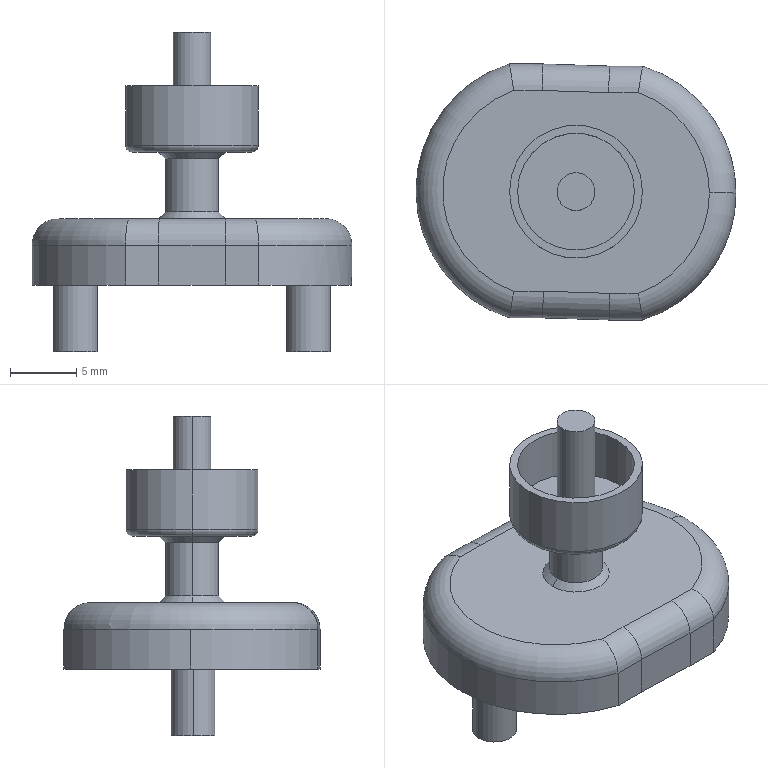Part | SolidWorks | features ICE 5, Fillet 2, Chamfer 1, Extrusion 1 | 1 solid | 44 faces | box 24.068 x 19.259 x 24 mm | volume 2234 mm3 | cylinder 21 | plane 14 | torus 5 | cone 4 | commonest cylinder face diameters 4 x8 3.305 x4 20 x3 2.85 x2 8.8 x2 10 x2
STEP:
#1=CARTESIAN_POINT('',(-1.721,5.002,10.));
#2=VERTEX_POINT('',#1);
#3=CARTESIAN_POINT('',(7.279,5.002,10.));
#4=VERTEX_POINT('',#3);
#5=CARTESIAN_POINT('',(2.779,5.002,10.));
#6=DIRECTION('',(0.,0.,-1.));
#7=DIRECTION('',(1.,0.,0.));
#8=AXIS2_PLACEMENT_3D('',#5,#6,#7);
#9=CIRCLE('',#8,4.5);
#10=EDGE_CURVE('',#2,#4,#9,.T.);
#11=ORIENTED_EDGE('',*,*,#10,.F.);
#12=CARTESIAN_POINT('',(-2.221,5.002,10.5));
#13=VERTEX_POINT('',#12);
#14=CARTESIAN_POINT('',(-1.721,5.002,10.5));
#15=DIRECTION('',(0.,1.,0.));
#16=DIRECTION('',(-1.,0.,0.));
#17=AXIS2_PLACEMENT_3D('',#14,#15,#16);
#18=CIRCLE('',#17,0.5);
#19=EDGE_CURVE('',#2,#13,#18,.T.);
#20=ORIENTED_EDGE('',*,*,#19,.T.);
#21=CARTESIAN_POINT('',(7.779,5.002,10.5));
#22=VERTEX_POINT('',#21);
#23=CARTESIAN_POINT('',(2.779,5.002,10.5));
#24=DIRECTION('',(0.,0.,1.));
#25=DIRECTION('',(1.,0.,0.));
#26=AXIS2_PLACEMENT_3D('',#23,#24,#25);
#27=CIRCLE('',#26,5.);
#28=EDGE_CURVE('',#22,#13,#27,.T.);
#29=ORIENTED_EDGE('',*,*,#28,.F.);
#30=CARTESIAN_POINT('',(7.279,5.002,10.5));
#31=DIRECTION('',(0.,-1.,0.));
#32=DIRECTION('',(0.,0.,-1.));
#33=AXIS2_PLACEMENT_3D('',#30,#31,#32);
#34=CIRCLE('',#33,0.5);
#35=EDGE_CURVE('',#4,#22,#34,.T.);
#36=ORIENTED_EDGE('',*,*,#35,.F.);
#37=EDGE_LOOP('',(#11,#20,#29,#36));
#38=FACE_OUTER_BOUND('',#37,.T.);
#39=CARTESIAN_POINT('',(2.779,5.002,10.5));
#40=DIRECTION('',(0.,0.,1.));
#41=DIRECTION('',(1.,0.,0.));
#42=AXIS2_PLACEMENT_3D('',#39,#40,#41);
#43=TOROIDAL_SURFACE('',#42,4.5,0.5);
#44=ADVANCED_FACE('',(#38),#43,.T.);
#45=CARTESIAN_POINT('',(4.779,5.002,5.5));
#46=VERTEX_POINT('',#45);
#47=CARTESIAN_POINT('',(0.7788,5.002,5.5));
#48=VERTEX_POINT('',#47);
#49=CARTESIAN_POINT('',(2.779,5.002,5.5));
#50=DIRECTION('',(0.,0.,1.));
#51=DIRECTION('',(1.,0.,0.));
#52=AXIS2_PLACEMENT_3D('',#49,#50,#51);
#53=CIRCLE('',#52,2.);
#54=EDGE_CURVE('',#46,#48,#53,.T.);
#55=ORIENTED_EDGE('',*,*,#54,.F.);
#56=CARTESIAN_POINT('',(5.279,5.002,5.));
#57=VERTEX_POINT('',#56);
#58=CARTESIAN_POINT('',(4.779,5.002,5.5));
#59=DIRECTION('',(0.7071,0.,-0.7071));
#60=VECTOR('',#59,1000.);
#61=LINE('',#58,#60);
#62=EDGE_CURVE('',#46,#57,#61,.T.);
#63=ORIENTED_EDGE('',*,*,#62,.T.);
#64=CARTESIAN_POINT('',(0.2788,5.002,5.));
#65=VERTEX_POINT('',#64);
#66=CARTESIAN_POINT('',(2.779,5.002,5.));
#67=DIRECTION('',(0.,0.,-1.));
#68=DIRECTION('',(1.,0.,0.));
#69=AXIS2_PLACEMENT_3D('',#66,#67,#68);
#70=CIRCLE('',#69,2.5);
#71=EDGE_CURVE('',#65,#57,#70,.T.);
#72=ORIENTED_EDGE('',*,*,#71,.F.);
#73=CARTESIAN_POINT('',(0.7788,5.002,5.5));
#74=DIRECTION('',(-0.7071,0.,-0.7071));
#75=VECTOR('',#74,1000.);
#76=LINE('',#73,#75);
#77=EDGE_CURVE('',#48,#65,#76,.T.);
#78=ORIENTED_EDGE('',*,*,#77,.F.);
#79=EDGE_LOOP('',(#55,#63,#72,#78));
#80=FACE_OUTER_BOUND('',#79,.T.);
#81=CARTESIAN_POINT('',(2.779,5.002,5.5));
#82=DIRECTION('',(0.,0.,-1.));
#83=DIRECTION('',(-1.,0.,0.));
#84=AXIS2_PLACEMENT_3D('',#81,#82,#83);
#85=CONICAL_SURFACE('',#84,2.,0.7854);
#86=ADVANCED_FACE('',(#80),#85,.T.);
#87=CARTESIAN_POINT('',(0.7788,5.002,9.5));
#88=VERTEX_POINT('',#87);
#89=CARTESIAN_POINT('',(4.779,5.002,9.5));
#90=VERTEX_POINT('',#89);
#91=CARTESIAN_POINT('',(2.779,5.002,9.5));
#92=DIRECTION('',(0.,0.,-1.));
#93=DIRECTION('',(1.,0.,0.));
#94=AXIS2_PLACEMENT_3D('',#91,#92,#93);
#95=CIRCLE('',#94,2.);
#96=EDGE_CURVE('',#88,#90,#95,.T.);
#97=ORIENTED_EDGE('',*,*,#96,.F.);
#98=CARTESIAN_POINT('',(0.2788,5.002,10.));
#99=VERTEX_POINT('',#98);
#100=CARTESIAN_POINT('',(0.2788,5.002,10.));
#101=DIRECTION('',(-0.7071,0.,0.7071));
#102=VECTOR('',#101,1000.);
#103=LINE('',#100,#102);
#104=EDGE_CURVE('',#88,#99,#103,.T.);
#105=ORIENTED_EDGE('',*,*,#104,.T.);
#106=CARTESIAN_POINT('',(5.279,5.002,10.));
#107=VERTEX_POINT('',#106);
#108=CARTESIAN_POINT('',(2.779,5.002,10.));
#109=DIRECTION('',(0.,0.,1.));
#110=DIRECTION('',(1.,0.,0.));
#111=AXIS2_PLACEMENT_3D('',#108,#109,#110);
#112=CIRCLE('',#111,2.5);
#113=EDGE_CURVE('',#107,#99,#112,.T.);
#114=ORIENTED_EDGE('',*,*,#113,.F.);
#115=CARTESIAN_POINT('',(5.279,5.002,10.));
#116=DIRECTION('',(0.7071,0.,0.7071));
#117=VECTOR('',#116,1000.);
#118=LINE('',#115,#117);
#119=EDGE_CURVE('',#90,#107,#118,.T.);
#120=ORIENTED_EDGE('',*,*,#119,.F.);
#121=EDGE_LOOP('',(#97,#105,#114,#120));
#122=FACE_OUTER_BOUND('',#121,.T.);
#123=CARTESIAN_POINT('',(2.779,5.002,10.));
#124=DIRECTION('',(0.,0.,1.));
#125=DIRECTION('',(1.,0.,0.));
#126=AXIS2_PLACEMENT_3D('',#123,#124,#125);
#127=CONICAL_SURFACE('',#126,2.5,0.7854);
#128=ADVANCED_FACE('',(#122),#127,.T.);
#129=CARTESIAN_POINT('',(4.204,5.002,19.));
#130=VERTEX_POINT('',#129);
#131=CARTESIAN_POINT('',(1.354,5.002,19.));
#132=VERTEX_POINT('',#131);
#133=CARTESIAN_POINT('',(2.779,5.002,19.));
#134=DIRECTION('',(0.,0.,1.));
#135=DIRECTION('',(1.,0.,0.));
#136=AXIS2_PLACEMENT_3D('',#133,#134,#135);
#137=CIRCLE('',#136,1.425);
#138=EDGE_CURVE('',#130,#132,#137,.T.);
#139=ORIENTED_EDGE('',*,*,#138,.F.);
#140=CARTESIAN_POINT('',(4.204,5.002,11.));
#141=VERTEX_POINT('',#140);
#142=CARTESIAN_POINT('',(4.204,5.002,19.));
#143=DIRECTION('',(0.,0.,-1.));
#144=VECTOR('',#143,1000.);
#145=LINE('',#142,#144);
#146=EDGE_CURVE('',#130,#141,#145,.T.);
#147=ORIENTED_EDGE('',*,*,#146,.T.);
#148=CARTESIAN_POINT('',(1.354,5.002,11.));
#149=VERTEX_POINT('',#148);
#150=CARTESIAN_POINT('',(2.779,5.002,11.));
#151=DIRECTION('',(0.,0.,1.));
#152=DIRECTION('',(1.,0.,0.));
#153=AXIS2_PLACEMENT_3D('',#150,#151,#152);
#154=CIRCLE('',#153,1.425);
#155=EDGE_CURVE('',#141,#149,#154,.T.);
#156=ORIENTED_EDGE('',*,*,#155,.T.);
#157=CARTESIAN_POINT('',(1.354,5.002,19.));
#158=DIRECTION('',(0.,0.,-1.));
#159=VECTOR('',#158,1000.);
#160=LINE('',#157,#159);
#161=EDGE_CURVE('',#132,#149,#160,.T.);
#162=ORIENTED_EDGE('',*,*,#161,.F.);
#163=EDGE_LOOP('',(#139,#147,#156,#162));
#164=FACE_OUTER_BOUND('',#163,.T.);
#165=CARTESIAN_POINT('',(2.779,5.002,19.));
#166=DIRECTION('',(0.,0.,-1.));
#167=DIRECTION('',(-1.,0.,0.));
#168=AXIS2_PLACEMENT_3D('',#165,#166,#167);
#169=CYLINDRICAL_SURFACE('',#168,1.425);
#170=ADVANCED_FACE('',(#164),#169,.T.);
#171=CARTESIAN_POINT('',(-1.621,5.002,15.));
#172=VERTEX_POINT('',#171);
#173=CARTESIAN_POINT('',(7.179,5.002,15.));
#174=VERTEX_POINT('',#173);
#175=CARTESIAN_POINT('',(2.779,5.002,15.));
#176=DIRECTION('',(0.,0.,1.));
#177=DIRECTION('',(1.,0.,0.));
#178=AXIS2_PLACEMENT_3D('',#175,#176,#177);
#179=CIRCLE('',#178,4.4);
#180=EDGE_CURVE('',#172,#174,#179,.T.);
#181=ORIENTED_EDGE('',*,*,#180,.T.);
#182=CARTESIAN_POINT('',(7.179,5.002,11.));
#183=VERTEX_POINT('',#182);
#184=CARTESIAN_POINT('',(7.179,5.002,15.));
#185=DIRECTION('',(0.,0.,-1.));
#186=VECTOR('',#185,1000.);
#187=LINE('',#184,#186);
#188=EDGE_CURVE('',#174,#183,#187,.T.);
#189=ORIENTED_EDGE('',*,*,#188,.T.);
#190=CARTESIAN_POINT('',(-1.621,5.002,11.));
#191=VERTEX_POINT('',#190);
#192=CARTESIAN_POINT('',(2.779,5.002,11.));
#193=DIRECTION('',(0.,0.,-1.));
#194=DIRECTION('',(1.,0.,0.));
#195=AXIS2_PLACEMENT_3D('',#192,#193,#194);
#196=CIRCLE('',#195,4.4);
#197=EDGE_CURVE('',#183,#191,#196,.T.);
#198=ORIENTED_EDGE('',*,*,#197,.T.);
#199=CARTESIAN_POINT('',(-1.621,5.002,15.));
#200=DIRECTION('',(0.,0.,-1.));
#201=VECTOR('',#200,1000.);
#202=LINE('',#199,#201);
#203=EDGE_CURVE('',#172,#191,#202,.T.);
#204=ORIENTED_EDGE('',*,*,#203,.F.);
#205=EDGE_LOOP('',(#181,#189,#198,#204));
#206=FACE_OUTER_BOUND('',#205,.T.);
#207=CARTESIAN_POINT('',(2.779,5.002,15.));
#208=DIRECTION('',(0.,0.,-1.));
#209=DIRECTION('',(-1.,0.,0.));
#210=AXIS2_PLACEMENT_3D('',#207,#208,#209);
#211=CYLINDRICAL_SURFACE('',#210,4.4);
#212=ADVANCED_FACE('',(#206),#211,.F.);
#213=CARTESIAN_POINT('',(7.779,5.002,15.));
#214=VERTEX_POINT('',#213);
#215=CARTESIAN_POINT('',(-2.221,5.002,15.));
#216=VERTEX_POINT('',#215);
#217=CARTESIAN_POINT('',(2.779,5.002,15.));
#218=DIRECTION('',(0.,0.,1.));
#219=DIRECTION('',(1.,0.,0.));
#220=AXIS2_PLACEMENT_3D('',#217,#218,#219);
#221=CIRCLE('',#220,5.);
#222=EDGE_CURVE('',#214,#216,#221,.T.);
#223=ORIENTED_EDGE('',*,*,#222,.F.);
#224=CARTESIAN_POINT('',(7.779,5.002,15.));
#225=DIRECTION('',(0.,0.,-1.));
#226=VECTOR('',#225,1000.);
#227=LINE('',#224,#226);
#228=EDGE_CURVE('',#214,#22,#227,.T.);
#229=ORIENTED_EDGE('',*,*,#228,.T.);
#230=ORIENTED_EDGE('',*,*,#28,.T.);
#231=CARTESIAN_POINT('',(-2.221,5.002,15.));
#232=DIRECTION('',(0.,0.,-1.));
#233=VECTOR('',#232,1000.);
#234=LINE('',#231,#233);
#235=EDGE_CURVE('',#216,#13,#234,.T.);
#236=ORIENTED_EDGE('',*,*,#235,.F.);
#237=EDGE_LOOP('',(#223,#229,#230,#236));
#238=FACE_OUTER_BOUND('',#237,.T.);
#239=CARTESIAN_POINT('',(2.779,5.002,15.));
#240=DIRECTION('',(0.,0.,-1.));
#241=DIRECTION('',(-1.,0.,0.));
#242=AXIS2_PLACEMENT_3D('',#239,#240,#241);
#243=CYLINDRICAL_SURFACE('',#242,5.);
#244=ADVANCED_FACE('',(#238),#243,.T.);
#245=ORIENTED_EDGE('',*,*,#96,.T.);
#246=CARTESIAN_POINT('',(4.779,5.002,10.));
#247=DIRECTION('',(0.,0.,-1.));
#248=VECTOR('',#247,1000.);
#249=LINE('',#246,#248);
#250=EDGE_CURVE('',#90,#46,#249,.T.);
#251=ORIENTED_EDGE('',*,*,#250,.T.);
#252=ORIENTED_EDGE('',*,*,#54,.T.);
#253=CARTESIAN_POINT('',(0.7788,5.002,10.));
#254=DIRECTION('',(0.,0.,-1.));
#255=VECTOR('',#254,1000.);
#256=LINE('',#253,#255);
#257=EDGE_CURVE('',#88,#48,#256,.T.);
#258=ORIENTED_EDGE('',*,*,#257,.F.);
#259=EDGE_LOOP('',(#245,#251,#252,#258));
#260=FACE_OUTER_BOUND('',#259,.T.);
#261=CARTESIAN_POINT('',(2.779,5.002,10.));
#262=DIRECTION('',(0.,0.,-1.));
#263=DIRECTION('',(-1.,0.,0.));
#264=AXIS2_PLACEMENT_3D('',#261,#262,#263);
#265=CYLINDRICAL_SURFACE('',#264,2.);
#266=ADVANCED_FACE('',(#260),#265,.T.);
#267=CARTESIAN_POINT('',(14.813,4.922,3.));
#268=VERTEX_POINT('',#267);
#269=CARTESIAN_POINT('',(7.779,-4.628,3.));
#270=VERTEX_POINT('',#269);
#271=CARTESIAN_POINT('',(4.813,4.922,3.));
#272=DIRECTION('',(0.,0.,-1.));
#273=DIRECTION('',(1.,0.,0.));
#274=AXIS2_PLACEMENT_3D('',#271,#272,#273);
#275=CIRCLE('',#274,10.);
#276=EDGE_CURVE('',#268,#270,#275,.T.);
#277=ORIENTED_EDGE('',*,*,#276,.F.);
#278=CARTESIAN_POINT('',(12.813,4.922,5.));
#279=VERTEX_POINT('',#278);
#280=CARTESIAN_POINT('',(12.813,4.922,3.));
#281=DIRECTION('',(0.,-1.,0.));
#282=DIRECTION('',(0.,0.,-1.));
#283=AXIS2_PLACEMENT_3D('',#280,#281,#282);
#284=CIRCLE('',#283,2.);
#285=EDGE_CURVE('',#268,#279,#284,.T.);
#286=ORIENTED_EDGE('',*,*,#285,.T.);
#287=CARTESIAN_POINT('',(7.458,-2.628,5.));
#288=VERTEX_POINT('',#287);
#289=CARTESIAN_POINT('',(4.813,4.922,5.));
#290=DIRECTION('',(0.,0.,1.));
#291=DIRECTION('',(1.,0.,0.));
#292=AXIS2_PLACEMENT_3D('',#289,#290,#291);
#293=CIRCLE('',#292,8.);
#294=EDGE_CURVE('',#288,#279,#293,.T.);
#295=ORIENTED_EDGE('',*,*,#294,.F.);
#296=CARTESIAN_POINT('',(7.779,-4.628,3.));
#297=CARTESIAN_POINT('',(7.779,-4.628,3.133));
#298=CARTESIAN_POINT('',(7.777,-4.614,3.264));
#299=CARTESIAN_POINT('',(7.769,-4.563,3.521));
#300=CARTESIAN_POINT('',(7.763,-4.524,3.648));
#301=CARTESIAN_POINT('',(7.748,-4.423,3.891));
#302=CARTESIAN_POINT('',(7.738,-4.361,4.006));
#303=CARTESIAN_POINT('',(7.716,-4.215,4.224));
#304=CARTESIAN_POINT('',(7.702,-4.13,4.327));
#305=CARTESIAN_POINT('',(7.659,-3.852,4.602));
#306=CARTESIAN_POINT('',(7.624,-3.629,4.75));
#307=CARTESIAN_POINT('',(7.546,-3.15,4.948));
#308=CARTESIAN_POINT('',(7.502,-2.886,5.));
#309=CARTESIAN_POINT('',(7.458,-2.628,5.));
#310=B_SPLINE_CURVE_WITH_KNOTS('',3,(#296,#297,#298,#299,#300,#301,#302,#303,#304,#305,#306,#307,#308,#309),.UNSPECIFIED.,.F.,.F.,(4,2,2,2,2,2,4),(0.,0.0003931,0.0007862,0.001179,0.001572,0.002359,0.003145),.UNSPECIFIED.);
#311=EDGE_CURVE('',#270,#288,#310,.T.);
#312=ORIENTED_EDGE('',*,*,#311,.F.);
#313=EDGE_LOOP('',(#277,#286,#295,#312));
#314=FACE_OUTER_BOUND('',#313,.T.);
#315=CARTESIAN_POINT('',(4.813,4.922,3.));
#316=DIRECTION('',(0.,0.,1.));
#317=DIRECTION('',(1.,0.,0.));
#318=AXIS2_PLACEMENT_3D('',#315,#316,#317);
#319=TOROIDAL_SURFACE('',#318,8.,2.);
#320=ADVANCED_FACE('',(#314),#319,.T.);
#321=CARTESIAN_POINT('',(-7.628,4.922,-5.));
#322=VERTEX_POINT('',#321);
#323=CARTESIAN_POINT('',(-4.323,4.922,-5.));
#324=VERTEX_POINT('',#323);
#325=CARTESIAN_POINT('',(-5.975,4.922,-5.));
#326=DIRECTION('',(0.,0.,-1.));
#327=DIRECTION('',(-1.,0.,0.));
#328=AXIS2_PLACEMENT_3D('',#325,#326,#327);
#329=CIRCLE('',#328,1.652);
#330=EDGE_CURVE('',#322,#324,#329,.T.);
#331=ORIENTED_EDGE('',*,*,#330,.F.);
#332=CARTESIAN_POINT('',(-7.628,4.922,0.));
#333=VERTEX_POINT('',#332);
#334=CARTESIAN_POINT('',(-7.628,4.922,-5.));
#335=DIRECTION('',(0.,0.,1.));
#336=VECTOR('',#335,1000.);
#337=LINE('',#334,#336);
#338=EDGE_CURVE('',#322,#333,#337,.T.);
#339=ORIENTED_EDGE('',*,*,#338,.T.);
#340=CARTESIAN_POINT('',(-4.323,4.922,0.));
#341=VERTEX_POINT('',#340);
#342=CARTESIAN_POINT('',(-5.975,4.922,0.));
#343=DIRECTION('',(0.,0.,-1.));
#344=DIRECTION('',(1.,0.,0.));
#345=AXIS2_PLACEMENT_3D('',#342,#343,#344);
#346=CIRCLE('',#345,1.652);
#347=EDGE_CURVE('',#333,#341,#346,.T.);
#348=ORIENTED_EDGE('',*,*,#347,.T.);
#349=CARTESIAN_POINT('',(-4.323,4.922,-5.));
#350=DIRECTION('',(0.,0.,1.));
#351=VECTOR('',#350,1000.);
#352=LINE('',#349,#351);
#353=EDGE_CURVE('',#324,#341,#352,.T.);
#354=ORIENTED_EDGE('',*,*,#353,.F.);
#355=EDGE_LOOP('',(#331,#339,#348,#354));
#356=FACE_OUTER_BOUND('',#355,.T.);
#357=CARTESIAN_POINT('',(-5.975,4.922,-5.));
#358=DIRECTION('',(0.,0.,1.));
#359=DIRECTION('',(1.,0.,0.));
#360=AXIS2_PLACEMENT_3D('',#357,#358,#359);
#361=CYLINDRICAL_SURFACE('',#360,1.652);
#362=ADVANCED_FACE('',(#356),#361,.T.);
#363=CARTESIAN_POINT('',(9.88,4.922,-5.));
#364=VERTEX_POINT('',#363);
#365=CARTESIAN_POINT('',(13.185,4.922,-5.));
#366=VERTEX_POINT('',#365);
#367=CARTESIAN_POINT('',(11.533,4.922,-5.));
#368=DIRECTION('',(0.,0.,-1.));
#369=DIRECTION('',(-1.,0.,0.));
#370=AXIS2_PLACEMENT_3D('',#367,#368,#369);
#371=CIRCLE('',#370,1.652);
#372=EDGE_CURVE('',#364,#366,#371,.T.);
#373=ORIENTED_EDGE('',*,*,#372,.F.);
#374=CARTESIAN_POINT('',(9.88,4.922,0.));
#375=VERTEX_POINT('',#374);
#376=CARTESIAN_POINT('',(9.88,4.922,-5.));
#377=DIRECTION('',(0.,0.,1.));
#378=VECTOR('',#377,1000.);
#379=LINE('',#376,#378);
#380=EDGE_CURVE('',#364,#375,#379,.T.);
#381=ORIENTED_EDGE('',*,*,#380,.T.);
#382=CARTESIAN_POINT('',(13.185,4.922,0.));
#383=VERTEX_POINT('',#382);
#384=CARTESIAN_POINT('',(11.533,4.922,0.));
#385=DIRECTION('',(0.,0.,-1.));
#386=DIRECTION('',(1.,0.,0.));
#387=AXIS2_PLACEMENT_3D('',#384,#385,#386);
#388=CIRCLE('',#387,1.652);
#389=EDGE_CURVE('',#375,#383,#388,.T.);
#390=ORIENTED_EDGE('',*,*,#389,.T.);
#391=CARTESIAN_POINT('',(13.185,4.922,-5.));
#392=DIRECTION('',(0.,0.,1.));
#393=VECTOR('',#392,1000.);
#394=LINE('',#391,#393);
#395=EDGE_CURVE('',#366,#383,#394,.T.);
#396=ORIENTED_EDGE('',*,*,#395,.F.);
#397=EDGE_LOOP('',(#373,#381,#390,#396));
#398=FACE_OUTER_BOUND('',#397,.T.);
#399=CARTESIAN_POINT('',(11.533,4.922,-5.));
#400=DIRECTION('',(0.,0.,1.));
#401=DIRECTION('',(1.,0.,0.));
#402=AXIS2_PLACEMENT_3D('',#399,#400,#401);
#403=CYLINDRICAL_SURFACE('',#402,1.652);
#404=ADVANCED_FACE('',(#398),#403,.T.);
#405=CARTESIAN_POINT('',(-2.221,-4.469,3.));
#406=VERTEX_POINT('',#405);
#407=CARTESIAN_POINT('',(-9.255,5.081,3.));
#408=VERTEX_POINT('',#407);
#409=CARTESIAN_POINT('',(0.7449,5.081,3.));
#410=DIRECTION('',(0.,0.,-1.));
#411=DIRECTION('',(1.,0.,0.));
#412=AXIS2_PLACEMENT_3D('',#409,#410,#411);
#413=CIRCLE('',#412,10.);
#414=EDGE_CURVE('',#406,#408,#413,.T.);
#415=ORIENTED_EDGE('',*,*,#414,.T.);
#416=CARTESIAN_POINT('',(-9.255,5.081,0.));
#417=VERTEX_POINT('',#416);
#418=CARTESIAN_POINT('',(-9.255,5.081,5.));
#419=DIRECTION('',(0.,0.,-1.));
#420=VECTOR('',#419,1000.);
#421=LINE('',#418,#420);
#422=EDGE_CURVE('',#408,#417,#421,.T.);
#423=ORIENTED_EDGE('',*,*,#422,.T.);
#424=CARTESIAN_POINT('',(-2.221,-4.469,0.));
#425=VERTEX_POINT('',#424);
#426=CARTESIAN_POINT('',(0.7449,5.081,0.));
#427=DIRECTION('',(0.,0.,1.));
#428=DIRECTION('',(1.,0.,0.));
#429=AXIS2_PLACEMENT_3D('',#426,#427,#428);
#430=CIRCLE('',#429,10.);
#431=EDGE_CURVE('',#417,#425,#430,.T.);
#432=ORIENTED_EDGE('',*,*,#431,.T.);
#433=CARTESIAN_POINT('',(-2.221,-4.469,5.));
#434=DIRECTION('',(0.,0.,-1.));
#435=VECTOR('',#434,1000.);
#436=LINE('',#433,#435);
#437=EDGE_CURVE('',#406,#425,#436,.T.);
#438=ORIENTED_EDGE('',*,*,#437,.F.);
#439=EDGE_LOOP('',(#415,#423,#432,#438));
#440=FACE_OUTER_BOUND('',#439,.T.);
#441=CARTESIAN_POINT('',(0.7449,5.081,5.));
#442=DIRECTION('',(0.,0.,-1.));
#443=DIRECTION('',(-1.,0.,0.));
#444=AXIS2_PLACEMENT_3D('',#441,#442,#443);
#445=CYLINDRICAL_SURFACE('',#444,10.);
#446=ADVANCED_FACE('',(#440),#445,.T.);
#447=CARTESIAN_POINT('',(0.2788,-4.469,3.));
#448=VERTEX_POINT('',#447);
#449=CARTESIAN_POINT('',(0.2788,-4.469,0.));
#450=VERTEX_POINT('',#449);
#451=CARTESIAN_POINT('',(0.2788,-4.469,5.));
#452=DIRECTION('',(0.,0.,-1.));
#453=VECTOR('',#452,1000.);
#454=LINE('',#451,#453);
#455=EDGE_CURVE('',#448,#450,#454,.T.);
#456=ORIENTED_EDGE('',*,*,#455,.F.);
#457=CARTESIAN_POINT('',(-2.221,-4.469,3.));
#458=DIRECTION('',(-1.,0.,0.));
#459=VECTOR('',#458,1000.);
#460=LINE('',#457,#459);
#461=EDGE_CURVE('',#448,#406,#460,.T.);
#462=ORIENTED_EDGE('',*,*,#461,.T.);
#463=ORIENTED_EDGE('',*,*,#437,.T.);
#464=CARTESIAN_POINT('',(-1.721,-4.469,0.));
#465=DIRECTION('',(1.,0.,0.));
#466=VECTOR('',#465,1000.);
#467=LINE('',#464,#466);
#468=EDGE_CURVE('',#425,#450,#467,.T.);
#469=ORIENTED_EDGE('',*,*,#468,.T.);
#470=EDGE_LOOP('',(#456,#462,#463,#469));
#471=FACE_OUTER_BOUND('',#470,.T.);
#472=CARTESIAN_POINT('',(-1.721,-4.469,5.));
#473=DIRECTION('',(0.,1.,0.));
#474=DIRECTION('',(0.,0.,1.));
#475=AXIS2_PLACEMENT_3D('',#472,#473,#474);
#476=PLANE('',#475);
#477=ADVANCED_FACE('',(#471),#476,.F.);
#478=CARTESIAN_POINT('',(5.279,-4.628,3.));
#479=VERTEX_POINT('',#478);
#480=CARTESIAN_POINT('',(5.279,-4.628,0.));
#481=VERTEX_POINT('',#480);
#482=CARTESIAN_POINT('',(5.279,-4.628,5.));
#483=DIRECTION('',(0.,0.,-1.));
#484=VECTOR('',#483,1000.);
#485=LINE('',#482,#484);
#486=EDGE_CURVE('',#479,#481,#485,.T.);
#487=ORIENTED_EDGE('',*,*,#486,.F.);
#488=CARTESIAN_POINT('',(0.2788,-4.469,3.));
#489=DIRECTION('',(-0.9995,0.03174,0.));
#490=VECTOR('',#489,1000.);
#491=LINE('',#488,#490);
#492=EDGE_CURVE('',#479,#448,#491,.T.);
#493=ORIENTED_EDGE('',*,*,#492,.T.);
#494=ORIENTED_EDGE('',*,*,#455,.T.);
#495=CARTESIAN_POINT('',(5.279,-4.628,0.));
#496=DIRECTION('',(0.9995,-0.03174,0.));
#497=VECTOR('',#496,1000.);
#498=LINE('',#495,#497);
#499=EDGE_CURVE('',#450,#481,#498,.T.);
#500=ORIENTED_EDGE('',*,*,#499,.T.);
#501=EDGE_LOOP('',(#487,#493,#494,#500));
#502=FACE_OUTER_BOUND('',#501,.T.);
#503=CARTESIAN_POINT('',(5.279,-4.628,5.));
#504=DIRECTION('',(0.03174,0.9995,0.));
#505=DIRECTION('',(-0.9995,0.03174,0.));
#506=AXIS2_PLACEMENT_3D('',#503,#504,#505);
#507=PLANE('',#506);
#508=ADVANCED_FACE('',(#502),#507,.F.);
#509=CARTESIAN_POINT('',(7.779,-4.628,0.));
#510=VERTEX_POINT('',#509);
#511=CARTESIAN_POINT('',(7.779,-4.628,5.));
#512=DIRECTION('',(0.,0.,-1.));
#513=VECTOR('',#512,1000.);
#514=LINE('',#511,#513);
#515=EDGE_CURVE('',#270,#510,#514,.T.);
#516=ORIENTED_EDGE('',*,*,#515,.F.);
#517=CARTESIAN_POINT('',(5.279,-4.628,3.));
#518=DIRECTION('',(-1.,0.,0.));
#519=VECTOR('',#518,1000.);
#520=LINE('',#517,#519);
#521=EDGE_CURVE('',#270,#479,#520,.T.);
#522=ORIENTED_EDGE('',*,*,#521,.T.);
#523=ORIENTED_EDGE('',*,*,#486,.T.);
#524=CARTESIAN_POINT('',(7.779,-4.628,0.));
#525=DIRECTION('',(1.,0.,0.));
#526=VECTOR('',#525,1000.);
#527=LINE('',#524,#526);
#528=EDGE_CURVE('',#481,#510,#527,.T.);
#529=ORIENTED_EDGE('',*,*,#528,.T.);
#530=EDGE_LOOP('',(#516,#522,#523,#529));
#531=FACE_OUTER_BOUND('',#530,.T.);
#532=CARTESIAN_POINT('',(7.779,-4.628,5.));
#533=DIRECTION('',(0.,1.,0.));
#534=DIRECTION('',(0.,0.,1.));
#535=AXIS2_PLACEMENT_3D('',#532,#533,#534);
#536=PLANE('',#535);
#537=ADVANCED_FACE('',(#531),#536,.F.);
#538=CARTESIAN_POINT('',(7.779,14.472,3.));
#539=VERTEX_POINT('',#538);
#540=CARTESIAN_POINT('',(7.779,14.472,0.));
#541=VERTEX_POINT('',#540);
#542=CARTESIAN_POINT('',(7.779,14.472,5.));
#543=DIRECTION('',(0.,0.,-1.));
#544=VECTOR('',#543,1000.);
#545=LINE('',#542,#544);
#546=EDGE_CURVE('',#539,#541,#545,.T.);
#547=ORIENTED_EDGE('',*,*,#546,.F.);
#548=CARTESIAN_POINT('',(4.813,4.922,3.));
#549=DIRECTION('',(0.,0.,-1.));
#550=DIRECTION('',(1.,0.,0.));
#551=AXIS2_PLACEMENT_3D('',#548,#549,#550);
#552=CIRCLE('',#551,10.);
#553=EDGE_CURVE('',#539,#268,#552,.T.);
#554=ORIENTED_EDGE('',*,*,#553,.T.);
#555=ORIENTED_EDGE('',*,*,#276,.T.);
#556=ORIENTED_EDGE('',*,*,#515,.T.);
#557=CARTESIAN_POINT('',(4.813,4.922,0.));
#558=DIRECTION('',(0.,0.,1.));
#559=DIRECTION('',(1.,0.,0.));
#560=AXIS2_PLACEMENT_3D('',#557,#558,#559);
#561=CIRCLE('',#560,10.);
#562=EDGE_CURVE('',#510,#541,#561,.T.);
#563=ORIENTED_EDGE('',*,*,#562,.T.);
#564=EDGE_LOOP('',(#547,#554,#555,#556,#563));
#565=FACE_OUTER_BOUND('',#564,.T.);
#566=CARTESIAN_POINT('',(4.813,4.922,5.));
#567=DIRECTION('',(0.,0.,-1.));
#568=DIRECTION('',(-1.,0.,0.));
#569=AXIS2_PLACEMENT_3D('',#566,#567,#568);
#570=CYLINDRICAL_SURFACE('',#569,10.);
#571=ADVANCED_FACE('',(#565),#570,.T.);
#572=CARTESIAN_POINT('',(5.279,14.472,3.));
#573=VERTEX_POINT('',#572);
#574=CARTESIAN_POINT('',(5.279,14.472,0.));
#575=VERTEX_POINT('',#574);
#576=CARTESIAN_POINT('',(5.279,14.472,5.));
#577=DIRECTION('',(0.,0.,-1.));
#578=VECTOR('',#577,1000.);
#579=LINE('',#576,#578);
#580=EDGE_CURVE('',#573,#575,#579,.T.);
#581=ORIENTED_EDGE('',*,*,#580,.F.);
#582=CARTESIAN_POINT('',(7.779,14.472,3.));
#583=DIRECTION('',(1.,0.,0.));
#584=VECTOR('',#583,1000.);
#585=LINE('',#582,#584);
#586=EDGE_CURVE('',#573,#539,#585,.T.);
#587=ORIENTED_EDGE('',*,*,#586,.T.);
#588=ORIENTED_EDGE('',*,*,#546,.T.);
#589=CARTESIAN_POINT('',(7.279,14.472,0.));
#590=DIRECTION('',(-1.,0.,0.));
#591=VECTOR('',#590,1000.);
#592=LINE('',#589,#591);
#593=EDGE_CURVE('',#541,#575,#592,.T.);
#594=ORIENTED_EDGE('',*,*,#593,.T.);
#595=EDGE_LOOP('',(#581,#587,#588,#594));
#596=FACE_OUTER_BOUND('',#595,.T.);
#597=CARTESIAN_POINT('',(7.279,14.472,5.));
#598=DIRECTION('',(0.,-1.,0.));
#599=DIRECTION('',(0.,0.,-1.));
#600=AXIS2_PLACEMENT_3D('',#597,#598,#599);
#601=PLANE('',#600);
#602=ADVANCED_FACE('',(#596),#601,.F.);
#603=CARTESIAN_POINT('',(0.2788,14.631,3.));
#604=VERTEX_POINT('',#603);
#605=CARTESIAN_POINT('',(0.2788,14.631,0.));
#606=VERTEX_POINT('',#605);
#607=CARTESIAN_POINT('',(0.2788,14.631,5.));
#608=DIRECTION('',(0.,0.,-1.));
#609=VECTOR('',#608,1000.);
#610=LINE('',#607,#609);
#611=EDGE_CURVE('',#604,#606,#610,.T.);
#612=ORIENTED_EDGE('',*,*,#611,.F.);
#613=CARTESIAN_POINT('',(5.279,14.472,3.));
#614=DIRECTION('',(0.9995,-0.03174,0.));
#615=VECTOR('',#614,1000.);
#616=LINE('',#613,#615);
#617=EDGE_CURVE('',#604,#573,#616,.T.);
#618=ORIENTED_EDGE('',*,*,#617,.T.);
#619=ORIENTED_EDGE('',*,*,#580,.T.);
#620=CARTESIAN_POINT('',(0.2788,14.631,0.));
#621=DIRECTION('',(-0.9995,0.03174,0.));
#622=VECTOR('',#621,1000.);
#623=LINE('',#620,#622);
#624=EDGE_CURVE('',#575,#606,#623,.T.);
#625=ORIENTED_EDGE('',*,*,#624,.T.);
#626=EDGE_LOOP('',(#612,#618,#619,#625));
#627=FACE_OUTER_BOUND('',#626,.T.);
#628=CARTESIAN_POINT('',(0.2788,14.631,5.));
#629=DIRECTION('',(-0.03174,-0.9995,0.));
#630=DIRECTION('',(0.9995,-0.03174,0.));
#631=AXIS2_PLACEMENT_3D('',#628,#629,#630);
#632=PLANE('',#631);
#633=ADVANCED_FACE('',(#627),#632,.F.);
#634=CARTESIAN_POINT('',(-2.221,14.631,3.));
#635=VERTEX_POINT('',#634);
#636=CARTESIAN_POINT('',(-2.221,14.631,0.));
#637=VERTEX_POINT('',#636);
#638=CARTESIAN_POINT('',(-2.221,14.631,5.));
#639=DIRECTION('',(0.,0.,-1.));
#640=VECTOR('',#639,1000.);
#641=LINE('',#638,#640);
#642=EDGE_CURVE('',#635,#637,#641,.T.);
#643=ORIENTED_EDGE('',*,*,#642,.F.);
#644=CARTESIAN_POINT('',(0.2788,14.631,3.));
#645=DIRECTION('',(1.,0.,0.));
#646=VECTOR('',#645,1000.);
#647=LINE('',#644,#646);
#648=EDGE_CURVE('',#635,#604,#647,.T.);
#649=ORIENTED_EDGE('',*,*,#648,.T.);
#650=ORIENTED_EDGE('',*,*,#611,.T.);
#651=CARTESIAN_POINT('',(-2.221,14.631,0.));
#652=DIRECTION('',(-1.,0.,0.));
#653=VECTOR('',#652,1000.);
#654=LINE('',#651,#653);
#655=EDGE_CURVE('',#606,#637,#654,.T.);
#656=ORIENTED_EDGE('',*,*,#655,.T.);
#657=EDGE_LOOP('',(#643,#649,#650,#656));
#658=FACE_OUTER_BOUND('',#657,.T.);
#659=CARTESIAN_POINT('',(-2.221,14.631,5.));
#660=DIRECTION('',(0.,-1.,0.));
#661=DIRECTION('',(0.,0.,-1.));
#662=AXIS2_PLACEMENT_3D('',#659,#660,#661);
#663=PLANE('',#662);
#664=ADVANCED_FACE('',(#658),#663,.F.);
#665=ORIENTED_EDGE('',*,*,#422,.F.);
#666=CARTESIAN_POINT('',(0.7449,5.081,3.));
#667=DIRECTION('',(0.,0.,-1.));
#668=DIRECTION('',(1.,0.,0.));
#669=AXIS2_PLACEMENT_3D('',#666,#667,#668);
#670=CIRCLE('',#669,10.);
#671=EDGE_CURVE('',#408,#635,#670,.T.);
#672=ORIENTED_EDGE('',*,*,#671,.T.);
#673=ORIENTED_EDGE('',*,*,#642,.T.);
#674=CARTESIAN_POINT('',(0.7449,5.081,0.));
#675=DIRECTION('',(0.,0.,1.));
#676=DIRECTION('',(1.,0.,0.));
#677=AXIS2_PLACEMENT_3D('',#674,#675,#676);
#678=CIRCLE('',#677,10.);
#679=EDGE_CURVE('',#637,#417,#678,.T.);
#680=ORIENTED_EDGE('',*,*,#679,.T.);
#681=EDGE_LOOP('',(#665,#672,#673,#680));
#682=FACE_OUTER_BOUND('',#681,.T.);
#683=CARTESIAN_POINT('',(0.7449,5.081,5.));
#684=DIRECTION('',(0.,0.,-1.));
#685=DIRECTION('',(-1.,0.,0.));
#686=AXIS2_PLACEMENT_3D('',#683,#684,#685);
#687=CYLINDRICAL_SURFACE('',#686,10.);
#688=ADVANCED_FACE('',(#682),#687,.T.);
#689=ORIENTED_EDGE('',*,*,#71,.T.);
#690=CARTESIAN_POINT('',(2.779,5.002,5.));
#691=DIRECTION('',(0.,0.,-1.));
#692=DIRECTION('',(1.,0.,0.));
#693=AXIS2_PLACEMENT_3D('',#690,#691,#692);
#694=CIRCLE('',#693,2.5);
#695=EDGE_CURVE('',#57,#65,#694,.T.);
#696=ORIENTED_EDGE('',*,*,#695,.T.);
#697=EDGE_LOOP('',(#689,#696));
#698=FACE_BOUND('',#697,.T.);
#699=CARTESIAN_POINT('',(0.247,12.631,5.));
#700=VERTEX_POINT('',#699);
#701=CARTESIAN_POINT('',(-1.9,12.631,5.));
#702=VERTEX_POINT('',#701);
#703=CARTESIAN_POINT('',(-2.221,12.631,5.));
#704=DIRECTION('',(-1.,0.,0.));
#705=VECTOR('',#704,1000.);
#706=LINE('',#703,#705);
#707=EDGE_CURVE('',#700,#702,#706,.T.);
#708=ORIENTED_EDGE('',*,*,#707,.T.);
#709=CARTESIAN_POINT('',(-1.9,-2.469,5.));
#710=VERTEX_POINT('',#709);
#711=CARTESIAN_POINT('',(0.7449,5.081,5.));
#712=DIRECTION('',(0.,0.,1.));
#713=DIRECTION('',(1.,0.,0.));
#714=AXIS2_PLACEMENT_3D('',#711,#712,#713);
#715=CIRCLE('',#714,8.);
#716=EDGE_CURVE('',#702,#710,#715,.T.);
#717=ORIENTED_EDGE('',*,*,#716,.T.);
#718=CARTESIAN_POINT('',(0.3105,-2.469,5.));
#719=VERTEX_POINT('',#718);
#720=CARTESIAN_POINT('',(0.2788,-2.469,5.));
#721=DIRECTION('',(1.,0.,0.));
#722=VECTOR('',#721,1000.);
#723=LINE('',#720,#722);
#724=EDGE_CURVE('',#710,#719,#723,.T.);
#725=ORIENTED_EDGE('',*,*,#724,.T.);
#726=CARTESIAN_POINT('',(5.311,-2.628,5.));
#727=VERTEX_POINT('',#726);
#728=CARTESIAN_POINT('',(5.342,-2.629,5.));
#729=DIRECTION('',(0.9995,-0.03174,0.));
#730=VECTOR('',#729,1000.);
#731=LINE('',#728,#730);
#732=EDGE_CURVE('',#719,#727,#731,.T.);
#733=ORIENTED_EDGE('',*,*,#732,.T.);
#734=CARTESIAN_POINT('',(7.779,-2.628,5.));
#735=DIRECTION('',(1.,0.,0.));
#736=VECTOR('',#735,1000.);
#737=LINE('',#734,#736);
#738=EDGE_CURVE('',#727,#288,#737,.T.);
#739=ORIENTED_EDGE('',*,*,#738,.T.);
#740=ORIENTED_EDGE('',*,*,#294,.T.);
#741=CARTESIAN_POINT('',(7.458,12.472,5.));
#742=VERTEX_POINT('',#741);
#743=CARTESIAN_POINT('',(4.813,4.922,5.));
#744=DIRECTION('',(0.,0.,1.));
#745=DIRECTION('',(1.,0.,0.));
#746=AXIS2_PLACEMENT_3D('',#743,#744,#745);
#747=CIRCLE('',#746,8.);
#748=EDGE_CURVE('',#279,#742,#747,.T.);
#749=ORIENTED_EDGE('',*,*,#748,.T.);
#750=CARTESIAN_POINT('',(5.247,12.472,5.));
#751=VERTEX_POINT('',#750);
#752=CARTESIAN_POINT('',(5.279,12.472,5.));
#753=DIRECTION('',(-1.,0.,0.));
#754=VECTOR('',#753,1000.);
#755=LINE('',#752,#754);
#756=EDGE_CURVE('',#742,#751,#755,.T.);
#757=ORIENTED_EDGE('',*,*,#756,.T.);
#758=CARTESIAN_POINT('',(0.2153,12.632,5.));
#759=DIRECTION('',(-0.9995,0.03174,0.));
#760=VECTOR('',#759,1000.);
#761=LINE('',#758,#760);
#762=EDGE_CURVE('',#751,#700,#761,.T.);
#763=ORIENTED_EDGE('',*,*,#762,.T.);
#764=EDGE_LOOP('',(#708,#717,#725,#733,#739,#740,#749,#757,#763));
#765=FACE_OUTER_BOUND('',#764,.T.);
#766=CARTESIAN_POINT('',(4.813,4.922,5.));
#767=DIRECTION('',(0.,0.,1.));
#768=DIRECTION('',(1.,0.,0.));
#769=AXIS2_PLACEMENT_3D('',#766,#767,#768);
#770=PLANE('',#769);
#771=ADVANCED_FACE('',(#698,#765),#770,.T.);
#772=CARTESIAN_POINT('',(-5.975,4.922,0.));
#773=DIRECTION('',(0.,0.,-1.));
#774=DIRECTION('',(1.,0.,0.));
#775=AXIS2_PLACEMENT_3D('',#772,#773,#774);
#776=CIRCLE('',#775,1.652);
#777=EDGE_CURVE('',#341,#333,#776,.T.);
#778=ORIENTED_EDGE('',*,*,#777,.F.);
#779=ORIENTED_EDGE('',*,*,#347,.F.);
#780=EDGE_LOOP('',(#778,#779));
#781=FACE_BOUND('',#780,.T.);
#782=CARTESIAN_POINT('',(11.533,4.922,0.));
#783=DIRECTION('',(0.,0.,-1.));
#784=DIRECTION('',(1.,0.,0.));
#785=AXIS2_PLACEMENT_3D('',#782,#783,#784);
#786=CIRCLE('',#785,1.652);
#787=EDGE_CURVE('',#383,#375,#786,.T.);
#788=ORIENTED_EDGE('',*,*,#787,.F.);
#789=ORIENTED_EDGE('',*,*,#389,.F.);
#790=EDGE_LOOP('',(#788,#789));
#791=FACE_BOUND('',#790,.T.);
#792=ORIENTED_EDGE('',*,*,#468,.F.);
#793=ORIENTED_EDGE('',*,*,#431,.F.);
#794=ORIENTED_EDGE('',*,*,#679,.F.);
#795=ORIENTED_EDGE('',*,*,#655,.F.);
#796=ORIENTED_EDGE('',*,*,#624,.F.);
#797=ORIENTED_EDGE('',*,*,#593,.F.);
#798=ORIENTED_EDGE('',*,*,#562,.F.);
#799=ORIENTED_EDGE('',*,*,#528,.F.);
#800=ORIENTED_EDGE('',*,*,#499,.F.);
#801=EDGE_LOOP('',(#792,#793,#794,#795,#796,#797,#798,#799,#800));
#802=FACE_OUTER_BOUND('',#801,.T.);
#803=CARTESIAN_POINT('',(4.813,4.922,0.));
#804=DIRECTION('',(0.,0.,1.));
#805=DIRECTION('',(1.,0.,0.));
#806=AXIS2_PLACEMENT_3D('',#803,#804,#805);
#807=PLANE('',#806);
#808=ADVANCED_FACE('',(#781,#791,#802),#807,.F.);
#809=ORIENTED_EDGE('',*,*,#380,.F.);
#810=CARTESIAN_POINT('',(11.533,4.922,-5.));
#811=DIRECTION('',(0.,0.,-1.));
#812=DIRECTION('',(-1.,0.,0.));
#813=AXIS2_PLACEMENT_3D('',#810,#811,#812);
#814=CIRCLE('',#813,1.652);
#815=EDGE_CURVE('',#366,#364,#814,.T.);
#816=ORIENTED_EDGE('',*,*,#815,.F.);
#817=ORIENTED_EDGE('',*,*,#395,.T.);
#818=ORIENTED_EDGE('',*,*,#787,.T.);
#819=EDGE_LOOP('',(#809,#816,#817,#818));
#820=FACE_OUTER_BOUND('',#819,.T.);
#821=CARTESIAN_POINT('',(11.533,4.922,-5.));
#822=DIRECTION('',(0.,0.,1.));
#823=DIRECTION('',(1.,0.,0.));
#824=AXIS2_PLACEMENT_3D('',#821,#822,#823);
#825=CYLINDRICAL_SURFACE('',#824,1.652);
#826=ADVANCED_FACE('',(#820),#825,.T.);
#827=ORIENTED_EDGE('',*,*,#815,.T.);
#828=ORIENTED_EDGE('',*,*,#372,.T.);
#829=EDGE_LOOP('',(#827,#828));
#830=FACE_OUTER_BOUND('',#829,.T.);
#831=CARTESIAN_POINT('',(11.533,4.922,-5.));
#832=DIRECTION('',(0.,0.,-1.));
#833=DIRECTION('',(-1.,0.,0.));
#834=AXIS2_PLACEMENT_3D('',#831,#832,#833);
#835=PLANE('',#834);
#836=ADVANCED_FACE('',(#830),#835,.T.);
#837=ORIENTED_EDGE('',*,*,#338,.F.);
#838=CARTESIAN_POINT('',(-5.975,4.922,-5.));
#839=DIRECTION('',(0.,0.,-1.));
#840=DIRECTION('',(-1.,0.,0.));
#841=AXIS2_PLACEMENT_3D('',#838,#839,#840);
#842=CIRCLE('',#841,1.652);
#843=EDGE_CURVE('',#324,#322,#842,.T.);
#844=ORIENTED_EDGE('',*,*,#843,.F.);
#845=ORIENTED_EDGE('',*,*,#353,.T.);
#846=ORIENTED_EDGE('',*,*,#777,.T.);
#847=EDGE_LOOP('',(#837,#844,#845,#846));
#848=FACE_OUTER_BOUND('',#847,.T.);
#849=CARTESIAN_POINT('',(-5.975,4.922,-5.));
#850=DIRECTION('',(0.,0.,1.));
#851=DIRECTION('',(1.,0.,0.));
#852=AXIS2_PLACEMENT_3D('',#849,#850,#851);
#853=CYLINDRICAL_SURFACE('',#852,1.652);
#854=ADVANCED_FACE('',(#848),#853,.T.);
#855=ORIENTED_EDGE('',*,*,#843,.T.);
#856=ORIENTED_EDGE('',*,*,#330,.T.);
#857=EDGE_LOOP('',(#855,#856));
#858=FACE_OUTER_BOUND('',#857,.T.);
#859=CARTESIAN_POINT('',(-5.975,4.922,-5.));
#860=DIRECTION('',(0.,0.,-1.));
#861=DIRECTION('',(-1.,0.,0.));
#862=AXIS2_PLACEMENT_3D('',#859,#860,#861);
#863=PLANE('',#862);
#864=ADVANCED_FACE('',(#858),#863,.T.);
#865=ORIENTED_EDGE('',*,*,#285,.F.);
#866=ORIENTED_EDGE('',*,*,#553,.F.);
#867=CARTESIAN_POINT('',(7.458,12.472,5.));
#868=CARTESIAN_POINT('',(7.502,12.733,5.));
#869=CARTESIAN_POINT('',(7.546,12.995,4.948));
#870=CARTESIAN_POINT('',(7.624,13.474,4.75));
#871=CARTESIAN_POINT('',(7.659,13.697,4.602));
#872=CARTESIAN_POINT('',(7.702,13.975,4.327));
#873=CARTESIAN_POINT('',(7.716,14.06,4.224));
#874=CARTESIAN_POINT('',(7.738,14.206,4.006));
#875=CARTESIAN_POINT('',(7.748,14.268,3.891));
#876=CARTESIAN_POINT('',(7.763,14.369,3.648));
#877=CARTESIAN_POINT('',(7.769,14.408,3.521));
#878=CARTESIAN_POINT('',(7.777,14.459,3.264));
#879=CARTESIAN_POINT('',(7.779,14.472,3.133));
#880=CARTESIAN_POINT('',(7.779,14.472,3.));
#881=B_SPLINE_CURVE_WITH_KNOTS('',3,(#867,#868,#869,#870,#871,#872,#873,#874,#875,#876,#877,#878,#879,#880),.UNSPECIFIED.,.F.,.F.,(4,2,2,2,2,2,4),(-0.00001555,0.0007767,0.001569,0.001965,0.002361,0.002757,0.003154),.UNSPECIFIED.);
#882=EDGE_CURVE('',#742,#539,#881,.T.);
#883=ORIENTED_EDGE('',*,*,#882,.F.);
#884=ORIENTED_EDGE('',*,*,#748,.F.);
#885=EDGE_LOOP('',(#865,#866,#883,#884));
#886=FACE_OUTER_BOUND('',#885,.T.);
#887=CARTESIAN_POINT('',(4.813,4.922,3.));
#888=DIRECTION('',(0.,0.,1.));
#889=DIRECTION('',(1.,0.,0.));
#890=AXIS2_PLACEMENT_3D('',#887,#888,#889);
#891=TOROIDAL_SURFACE('',#890,8.,2.);
#892=ADVANCED_FACE('',(#886),#891,.T.);
#893=ORIENTED_EDGE('',*,*,#882,.T.);
#894=ORIENTED_EDGE('',*,*,#586,.F.);
#895=CARTESIAN_POINT('',(5.247,12.472,5.));
#896=CARTESIAN_POINT('',(5.266,13.644,5.));
#897=CARTESIAN_POINT('',(5.279,14.472,4.172));
#898=CARTESIAN_POINT('',(5.279,14.472,3.));
#899=(BOUNDED_CURVE()B_SPLINE_CURVE(3,(#895,#896,#897,#898),.UNSPECIFIED.,.F.,.F.)B_SPLINE_CURVE_WITH_KNOTS((4,4),(1.571,3.142),.UNSPECIFIED.)CURVE()GEOMETRIC_REPRESENTATION_ITEM()RATIONAL_B_SPLINE_CURVE((1.,0.8047,0.8047,1.))REPRESENTATION_ITEM(''));
#900=EDGE_CURVE('',#751,#573,#899,.T.);
#901=ORIENTED_EDGE('',*,*,#900,.F.);
#902=ORIENTED_EDGE('',*,*,#756,.F.);
#903=EDGE_LOOP('',(#893,#894,#901,#902));
#904=FACE_OUTER_BOUND('',#903,.T.);
#905=CARTESIAN_POINT('',(4.813,12.472,3.));
#906=DIRECTION('',(1.,0.,0.));
#907=DIRECTION('',(0.,0.,-1.));
#908=AXIS2_PLACEMENT_3D('',#905,#906,#907);
#909=CYLINDRICAL_SURFACE('',#908,2.);
#910=ADVANCED_FACE('',(#904),#909,.T.);
#911=ORIENTED_EDGE('',*,*,#311,.T.);
#912=ORIENTED_EDGE('',*,*,#738,.F.);
#913=CARTESIAN_POINT('',(5.279,-4.628,3.));
#914=CARTESIAN_POINT('',(5.279,-4.628,4.172));
#915=CARTESIAN_POINT('',(5.292,-3.799,5.));
#916=CARTESIAN_POINT('',(5.311,-2.628,5.));
#917=(BOUNDED_CURVE()B_SPLINE_CURVE(3,(#913,#914,#915,#916),.UNSPECIFIED.,.F.,.F.)B_SPLINE_CURVE_WITH_KNOTS((4,4),(3.142,4.712),.UNSPECIFIED.)CURVE()GEOMETRIC_REPRESENTATION_ITEM()RATIONAL_B_SPLINE_CURVE((1.,0.8047,0.8047,1.))REPRESENTATION_ITEM(''));
#918=EDGE_CURVE('',#479,#727,#917,.T.);
#919=ORIENTED_EDGE('',*,*,#918,.F.);
#920=ORIENTED_EDGE('',*,*,#521,.F.);
#921=EDGE_LOOP('',(#911,#912,#919,#920));
#922=FACE_OUTER_BOUND('',#921,.T.);
#923=CARTESIAN_POINT('',(4.813,-2.628,3.));
#924=DIRECTION('',(-1.,0.,0.));
#925=DIRECTION('',(0.,0.,1.));
#926=AXIS2_PLACEMENT_3D('',#923,#924,#925);
#927=CYLINDRICAL_SURFACE('',#926,2.);
#928=ADVANCED_FACE('',(#922),#927,.T.);
#929=ORIENTED_EDGE('',*,*,#900,.T.);
#930=ORIENTED_EDGE('',*,*,#617,.F.);
#931=CARTESIAN_POINT('',(0.247,12.631,5.));
#932=CARTESIAN_POINT('',(0.2656,13.803,5.));
#933=CARTESIAN_POINT('',(0.2788,14.631,4.172));
#934=CARTESIAN_POINT('',(0.2788,14.631,3.));
#935=(BOUNDED_CURVE()B_SPLINE_CURVE(3,(#931,#932,#933,#934),.UNSPECIFIED.,.F.,.F.)B_SPLINE_CURVE_WITH_KNOTS((4,4),(1.571,3.142),.UNSPECIFIED.)CURVE()GEOMETRIC_REPRESENTATION_ITEM()RATIONAL_B_SPLINE_CURVE((1.,0.8047,0.8047,1.))REPRESENTATION_ITEM(''));
#936=EDGE_CURVE('',#700,#604,#935,.T.);
#937=ORIENTED_EDGE('',*,*,#936,.F.);
#938=ORIENTED_EDGE('',*,*,#762,.F.);
#939=EDGE_LOOP('',(#929,#930,#937,#938));
#940=FACE_OUTER_BOUND('',#939,.T.);
#941=CARTESIAN_POINT('',(5.053,12.479,3.));
#942=DIRECTION('',(0.9995,-0.03174,0.));
#943=DIRECTION('',(0.03174,0.9995,0.));
#944=AXIS2_PLACEMENT_3D('',#941,#942,#943);
#945=CYLINDRICAL_SURFACE('',#944,2.);
#946=ADVANCED_FACE('',(#940),#945,.T.);
#947=ORIENTED_EDGE('',*,*,#918,.T.);
#948=ORIENTED_EDGE('',*,*,#732,.F.);
#949=CARTESIAN_POINT('',(0.2788,-4.469,3.));
#950=CARTESIAN_POINT('',(0.2788,-4.469,4.172));
#951=CARTESIAN_POINT('',(0.2919,-3.64,5.));
#952=CARTESIAN_POINT('',(0.3105,-2.469,5.));
#953=(BOUNDED_CURVE()B_SPLINE_CURVE(3,(#949,#950,#951,#952),.UNSPECIFIED.,.F.,.F.)B_SPLINE_CURVE_WITH_KNOTS((4,4),(3.142,4.712),.UNSPECIFIED.)CURVE()GEOMETRIC_REPRESENTATION_ITEM()RATIONAL_B_SPLINE_CURVE((1.,0.8047,0.8047,1.))REPRESENTATION_ITEM(''));
#954=EDGE_CURVE('',#448,#719,#953,.T.);
#955=ORIENTED_EDGE('',*,*,#954,.F.);
#956=ORIENTED_EDGE('',*,*,#492,.F.);
#957=EDGE_LOOP('',(#947,#948,#955,#956));
#958=FACE_OUTER_BOUND('',#957,.T.);
#959=CARTESIAN_POINT('',(4.574,-2.604,3.));
#960=DIRECTION('',(-0.9995,0.03174,0.));
#961=DIRECTION('',(-0.03174,-0.9995,0.));
#962=AXIS2_PLACEMENT_3D('',#959,#960,#961);
#963=CYLINDRICAL_SURFACE('',#962,2.);
#964=ADVANCED_FACE('',(#958),#963,.T.);
#965=ORIENTED_EDGE('',*,*,#936,.T.);
#966=ORIENTED_EDGE('',*,*,#648,.F.);
#967=CARTESIAN_POINT('',(-1.9,12.631,5.));
#968=CARTESIAN_POINT('',(-1.945,12.892,5.));
#969=CARTESIAN_POINT('',(-1.988,13.154,4.948));
#970=CARTESIAN_POINT('',(-2.066,13.633,4.75));
#971=CARTESIAN_POINT('',(-2.101,13.856,4.602));
#972=CARTESIAN_POINT('',(-2.145,14.134,4.327));
#973=CARTESIAN_POINT('',(-2.158,14.218,4.224));
#974=CARTESIAN_POINT('',(-2.181,14.365,4.006));
#975=CARTESIAN_POINT('',(-2.19,14.427,3.891));
#976=CARTESIAN_POINT('',(-2.205,14.528,3.648));
#977=CARTESIAN_POINT('',(-2.211,14.567,3.521));
#978=CARTESIAN_POINT('',(-2.219,14.618,3.264));
#979=CARTESIAN_POINT('',(-2.221,14.631,3.133));
#980=CARTESIAN_POINT('',(-2.221,14.631,3.));
#981=B_SPLINE_CURVE_WITH_KNOTS('',3,(#967,#968,#969,#970,#971,#972,#973,#974,#975,#976,#977,#978,#979,#980),.UNSPECIFIED.,.F.,.F.,(4,2,2,2,2,2,4),(-0.00001555,0.0007767,0.001569,0.001965,0.002361,0.002757,0.003154),.UNSPECIFIED.);
#982=EDGE_CURVE('',#702,#635,#981,.T.);
#983=ORIENTED_EDGE('',*,*,#982,.F.);
#984=ORIENTED_EDGE('',*,*,#707,.F.);
#985=EDGE_LOOP('',(#965,#966,#983,#984));
#986=FACE_OUTER_BOUND('',#985,.T.);
#987=CARTESIAN_POINT('',(4.813,12.631,3.));
#988=DIRECTION('',(1.,0.,0.));
#989=DIRECTION('',(0.,0.,-1.));
#990=AXIS2_PLACEMENT_3D('',#987,#988,#989);
#991=CYLINDRICAL_SURFACE('',#990,2.);
#992=ADVANCED_FACE('',(#986),#991,.T.);
#993=ORIENTED_EDGE('',*,*,#954,.T.);
#994=ORIENTED_EDGE('',*,*,#724,.F.);
#995=CARTESIAN_POINT('',(-2.221,-4.469,3.));
#996=CARTESIAN_POINT('',(-2.221,-4.469,3.133));
#997=CARTESIAN_POINT('',(-2.219,-4.456,3.264));
#998=CARTESIAN_POINT('',(-2.211,-4.404,3.521));
#999=CARTESIAN_POINT('',(-2.205,-4.365,3.648));
#1000=CARTESIAN_POINT('',(-2.19,-4.264,3.891));
#1001=CARTESIAN_POINT('',(-2.181,-4.202,4.006));
#1002=CARTESIAN_POINT('',(-2.158,-4.056,4.224));
#1003=CARTESIAN_POINT('',(-2.145,-3.971,4.327));
#1004=CARTESIAN_POINT('',(-2.101,-3.694,4.602));
#1005=CARTESIAN_POINT('',(-2.066,-3.471,4.75));
#1006=CARTESIAN_POINT('',(-1.988,-2.991,4.948));
#1007=CARTESIAN_POINT('',(-1.944,-2.727,5.));
#1008=CARTESIAN_POINT('',(-1.9,-2.469,5.));
#1009=B_SPLINE_CURVE_WITH_KNOTS('',3,(#995,#996,#997,#998,#999,#1000,#1001,#1002,#1003,#1004,#1005,#1006,#1007,#1008),.UNSPECIFIED.,.F.,.F.,(4,2,2,2,2,2,4),(0.,0.0003931,0.0007862,0.001179,0.001572,0.002359,0.003145),.UNSPECIFIED.);
#1010=EDGE_CURVE('',#406,#710,#1009,.T.);
#1011=ORIENTED_EDGE('',*,*,#1010,.F.);
#1012=ORIENTED_EDGE('',*,*,#461,.F.);
#1013=EDGE_LOOP('',(#993,#994,#1011,#1012));
#1014=FACE_OUTER_BOUND('',#1013,.T.);
#1015=CARTESIAN_POINT('',(4.813,-2.469,3.));
#1016=DIRECTION('',(-1.,0.,0.));
#1017=DIRECTION('',(0.,0.,1.));
#1018=AXIS2_PLACEMENT_3D('',#1015,#1016,#1017);
#1019=CYLINDRICAL_SURFACE('',#1018,2.);
#1020=ADVANCED_FACE('',(#1014),#1019,.T.);
#1021=ORIENTED_EDGE('',*,*,#982,.T.);
#1022=ORIENTED_EDGE('',*,*,#671,.F.);
#1023=ORIENTED_EDGE('',*,*,#414,.F.);
#1024=ORIENTED_EDGE('',*,*,#1010,.T.);
#1025=ORIENTED_EDGE('',*,*,#716,.F.);
#1026=EDGE_LOOP('',(#1021,#1022,#1023,#1024,#1025));
#1027=FACE_OUTER_BOUND('',#1026,.T.);
#1028=CARTESIAN_POINT('',(0.7449,5.081,3.));
#1029=DIRECTION('',(0.,0.,1.));
#1030=DIRECTION('',(1.,0.,0.));
#1031=AXIS2_PLACEMENT_3D('',#1028,#1029,#1030);
#1032=TOROIDAL_SURFACE('',#1031,8.,2.);
#1033=ADVANCED_FACE('',(#1027),#1032,.T.);
#1034=ORIENTED_EDGE('',*,*,#250,.F.);
#1035=CARTESIAN_POINT('',(2.779,5.002,9.5));
#1036=DIRECTION('',(0.,0.,-1.));
#1037=DIRECTION('',(1.,0.,0.));
#1038=AXIS2_PLACEMENT_3D('',#1035,#1036,#1037);
#1039=CIRCLE('',#1038,2.);
#1040=EDGE_CURVE('',#90,#88,#1039,.T.);
#1041=ORIENTED_EDGE('',*,*,#1040,.T.);
#1042=ORIENTED_EDGE('',*,*,#257,.T.);
#1043=CARTESIAN_POINT('',(2.779,5.002,5.5));
#1044=DIRECTION('',(0.,0.,1.));
#1045=DIRECTION('',(1.,0.,0.));
#1046=AXIS2_PLACEMENT_3D('',#1043,#1044,#1045);
#1047=CIRCLE('',#1046,2.);
#1048=EDGE_CURVE('',#48,#46,#1047,.T.);
#1049=ORIENTED_EDGE('',*,*,#1048,.T.);
#1050=EDGE_LOOP('',(#1034,#1041,#1042,#1049));
#1051=FACE_OUTER_BOUND('',#1050,.T.);
#1052=CARTESIAN_POINT('',(2.779,5.002,10.));
#1053=DIRECTION('',(0.,0.,-1.));
#1054=DIRECTION('',(-1.,0.,0.));
#1055=AXIS2_PLACEMENT_3D('',#1052,#1053,#1054);
#1056=CYLINDRICAL_SURFACE('',#1055,2.);
#1057=ADVANCED_FACE('',(#1051),#1056,.T.);
#1058=CARTESIAN_POINT('',(2.779,5.002,10.));
#1059=DIRECTION('',(0.,0.,-1.));
#1060=DIRECTION('',(1.,0.,0.));
#1061=AXIS2_PLACEMENT_3D('',#1058,#1059,#1060);
#1062=CIRCLE('',#1061,4.5);
#1063=EDGE_CURVE('',#4,#2,#1062,.T.);
#1064=ORIENTED_EDGE('',*,*,#1063,.T.);
#1065=ORIENTED_EDGE('',*,*,#10,.T.);
#1066=EDGE_LOOP('',(#1064,#1065));
#1067=FACE_OUTER_BOUND('',#1066,.T.);
#1068=ORIENTED_EDGE('',*,*,#113,.T.);
#1069=CARTESIAN_POINT('',(2.779,5.002,10.));
#1070=DIRECTION('',(0.,0.,1.));
#1071=DIRECTION('',(1.,0.,0.));
#1072=AXIS2_PLACEMENT_3D('',#1069,#1070,#1071);
#1073=CIRCLE('',#1072,2.5);
#1074=EDGE_CURVE('',#99,#107,#1073,.T.);
#1075=ORIENTED_EDGE('',*,*,#1074,.T.);
#1076=EDGE_LOOP('',(#1068,#1075));
#1077=FACE_BOUND('',#1076,.T.);
#1078=CARTESIAN_POINT('',(2.779,5.002,10.));
#1079=DIRECTION('',(0.,0.,1.));
#1080=DIRECTION('',(1.,0.,0.));
#1081=AXIS2_PLACEMENT_3D('',#1078,#1079,#1080);
#1082=PLANE('',#1081);
#1083=ADVANCED_FACE('',(#1067,#1077),#1082,.F.);
#1084=CARTESIAN_POINT('',(2.779,5.002,15.));
#1085=DIRECTION('',(0.,0.,1.));
#1086=DIRECTION('',(1.,0.,0.));
#1087=AXIS2_PLACEMENT_3D('',#1084,#1085,#1086);
#1088=CIRCLE('',#1087,5.);
#1089=EDGE_CURVE('',#216,#214,#1088,.T.);
#1090=ORIENTED_EDGE('',*,*,#1089,.T.);
#1091=ORIENTED_EDGE('',*,*,#222,.T.);
#1092=EDGE_LOOP('',(#1090,#1091));
#1093=FACE_OUTER_BOUND('',#1092,.T.);
#1094=ORIENTED_EDGE('',*,*,#180,.F.);
#1095=CARTESIAN_POINT('',(2.779,5.002,15.));
#1096=DIRECTION('',(0.,0.,1.));
#1097=DIRECTION('',(1.,0.,0.));
#1098=AXIS2_PLACEMENT_3D('',#1095,#1096,#1097);
#1099=CIRCLE('',#1098,4.4);
#1100=EDGE_CURVE('',#174,#172,#1099,.T.);
#1101=ORIENTED_EDGE('',*,*,#1100,.F.);
#1102=EDGE_LOOP('',(#1094,#1101));
#1103=FACE_BOUND('',#1102,.T.);
#1104=CARTESIAN_POINT('',(2.779,5.002,15.));
#1105=DIRECTION('',(0.,0.,1.));
#1106=DIRECTION('',(1.,0.,0.));
#1107=AXIS2_PLACEMENT_3D('',#1104,#1105,#1106);
#1108=PLANE('',#1107);
#1109=ADVANCED_FACE('',(#1093,#1103),#1108,.T.);
#1110=ORIENTED_EDGE('',*,*,#228,.F.);
#1111=ORIENTED_EDGE('',*,*,#1089,.F.);
#1112=ORIENTED_EDGE('',*,*,#235,.T.);
#1113=CARTESIAN_POINT('',(2.779,5.002,10.5));
#1114=DIRECTION('',(0.,0.,1.));
#1115=DIRECTION('',(1.,0.,0.));
#1116=AXIS2_PLACEMENT_3D('',#1113,#1114,#1115);
#1117=CIRCLE('',#1116,5.);
#1118=EDGE_CURVE('',#13,#22,#1117,.T.);
#1119=ORIENTED_EDGE('',*,*,#1118,.T.);
#1120=EDGE_LOOP('',(#1110,#1111,#1112,#1119));
#1121=FACE_OUTER_BOUND('',#1120,.T.);
#1122=CARTESIAN_POINT('',(2.779,5.002,15.));
#1123=DIRECTION('',(0.,0.,-1.));
#1124=DIRECTION('',(-1.,0.,0.));
#1125=AXIS2_PLACEMENT_3D('',#1122,#1123,#1124);
#1126=CYLINDRICAL_SURFACE('',#1125,5.);
#1127=ADVANCED_FACE('',(#1121),#1126,.T.);
#1128=ORIENTED_EDGE('',*,*,#188,.F.);
#1129=ORIENTED_EDGE('',*,*,#1100,.T.);
#1130=ORIENTED_EDGE('',*,*,#203,.T.);
#1131=CARTESIAN_POINT('',(2.779,5.002,11.));
#1132=DIRECTION('',(0.,0.,-1.));
#1133=DIRECTION('',(1.,0.,0.));
#1134=AXIS2_PLACEMENT_3D('',#1131,#1132,#1133);
#1135=CIRCLE('',#1134,4.4);
#1136=EDGE_CURVE('',#191,#183,#1135,.T.);
#1137=ORIENTED_EDGE('',*,*,#1136,.T.);
#1138=EDGE_LOOP('',(#1128,#1129,#1130,#1137));
#1139=FACE_OUTER_BOUND('',#1138,.T.);
#1140=CARTESIAN_POINT('',(2.779,5.002,15.));
#1141=DIRECTION('',(0.,0.,-1.));
#1142=DIRECTION('',(-1.,0.,0.));
#1143=AXIS2_PLACEMENT_3D('',#1140,#1141,#1142);
#1144=CYLINDRICAL_SURFACE('',#1143,4.4);
#1145=ADVANCED_FACE('',(#1139),#1144,.F.);
#1146=CARTESIAN_POINT('',(2.779,5.002,11.));
#1147=DIRECTION('',(0.,0.,1.));
#1148=DIRECTION('',(1.,0.,0.));
#1149=AXIS2_PLACEMENT_3D('',#1146,#1147,#1148);
#1150=CIRCLE('',#1149,1.425);
#1151=EDGE_CURVE('',#149,#141,#1150,.T.);
#1152=ORIENTED_EDGE('',*,*,#1151,.F.);
#1153=ORIENTED_EDGE('',*,*,#155,.F.);
#1154=EDGE_LOOP('',(#1152,#1153));
#1155=FACE_BOUND('',#1154,.T.);
#1156=ORIENTED_EDGE('',*,*,#1136,.F.);
#1157=ORIENTED_EDGE('',*,*,#197,.F.);
#1158=EDGE_LOOP('',(#1156,#1157));
#1159=FACE_OUTER_BOUND('',#1158,.T.);
#1160=CARTESIAN_POINT('',(2.779,5.002,11.));
#1161=DIRECTION('',(0.,0.,1.));
#1162=DIRECTION('',(1.,0.,0.));
#1163=AXIS2_PLACEMENT_3D('',#1160,#1161,#1162);
#1164=PLANE('',#1163);
#1165=ADVANCED_FACE('',(#1155,#1159),#1164,.T.);
#1166=ORIENTED_EDGE('',*,*,#146,.F.);
#1167=CARTESIAN_POINT('',(2.779,5.002,19.));
#1168=DIRECTION('',(0.,0.,1.));
#1169=DIRECTION('',(1.,0.,0.));
#1170=AXIS2_PLACEMENT_3D('',#1167,#1168,#1169);
#1171=CIRCLE('',#1170,1.425);
#1172=EDGE_CURVE('',#132,#130,#1171,.T.);
#1173=ORIENTED_EDGE('',*,*,#1172,.F.);
#1174=ORIENTED_EDGE('',*,*,#161,.T.);
#1175=ORIENTED_EDGE('',*,*,#1151,.T.);
#1176=EDGE_LOOP('',(#1166,#1173,#1174,#1175));
#1177=FACE_OUTER_BOUND('',#1176,.T.);
#1178=CARTESIAN_POINT('',(2.779,5.002,19.));
#1179=DIRECTION('',(0.,0.,-1.));
#1180=DIRECTION('',(-1.,0.,0.));
#1181=AXIS2_PLACEMENT_3D('',#1178,#1179,#1180);
#1182=CYLINDRICAL_SURFACE('',#1181,1.425);
#1183=ADVANCED_FACE('',(#1177),#1182,.T.);
#1184=ORIENTED_EDGE('',*,*,#1172,.T.);
#1185=ORIENTED_EDGE('',*,*,#138,.T.);
#1186=EDGE_LOOP('',(#1184,#1185));
#1187=FACE_OUTER_BOUND('',#1186,.T.);
#1188=CARTESIAN_POINT('',(2.779,5.002,19.));
#1189=DIRECTION('',(0.,0.,1.));
#1190=DIRECTION('',(1.,0.,0.));
#1191=AXIS2_PLACEMENT_3D('',#1188,#1189,#1190);
#1192=PLANE('',#1191);
#1193=ADVANCED_FACE('',(#1187),#1192,.T.);
#1194=ORIENTED_EDGE('',*,*,#104,.F.);
#1195=ORIENTED_EDGE('',*,*,#1040,.F.);
#1196=ORIENTED_EDGE('',*,*,#119,.T.);
#1197=ORIENTED_EDGE('',*,*,#1074,.F.);
#1198=EDGE_LOOP('',(#1194,#1195,#1196,#1197));
#1199=FACE_OUTER_BOUND('',#1198,.T.);
#1200=CARTESIAN_POINT('',(2.779,5.002,10.));
#1201=DIRECTION('',(0.,0.,1.));
#1202=DIRECTION('',(1.,0.,0.));
#1203=AXIS2_PLACEMENT_3D('',#1200,#1201,#1202);
#1204=CONICAL_SURFACE('',#1203,2.5,0.7854);
#1205=ADVANCED_FACE('',(#1199),#1204,.T.);
#1206=ORIENTED_EDGE('',*,*,#62,.F.);
#1207=ORIENTED_EDGE('',*,*,#1048,.F.);
#1208=ORIENTED_EDGE('',*,*,#77,.T.);
#1209=ORIENTED_EDGE('',*,*,#695,.F.);
#1210=EDGE_LOOP('',(#1206,#1207,#1208,#1209));
#1211=FACE_OUTER_BOUND('',#1210,.T.);
#1212=CARTESIAN_POINT('',(2.779,5.002,5.5));
#1213=DIRECTION('',(0.,0.,-1.));
#1214=DIRECTION('',(-1.,0.,0.));
#1215=AXIS2_PLACEMENT_3D('',#1212,#1213,#1214);
#1216=CONICAL_SURFACE('',#1215,2.,0.7854);
#1217=ADVANCED_FACE('',(#1211),#1216,.T.);
#1218=ORIENTED_EDGE('',*,*,#19,.F.);
#1219=ORIENTED_EDGE('',*,*,#1063,.F.);
#1220=ORIENTED_EDGE('',*,*,#35,.T.);
#1221=ORIENTED_EDGE('',*,*,#1118,.F.);
#1222=EDGE_LOOP('',(#1218,#1219,#1220,#1221));
#1223=FACE_OUTER_BOUND('',#1222,.T.);
#1224=CARTESIAN_POINT('',(2.779,5.002,10.5));
#1225=DIRECTION('',(0.,0.,1.));
#1226=DIRECTION('',(1.,0.,0.));
#1227=AXIS2_PLACEMENT_3D('',#1224,#1225,#1226);
#1228=TOROIDAL_SURFACE('',#1227,4.5,0.5);
#1229=ADVANCED_FACE('',(#1223),#1228,.T.);
#1230=CLOSED_SHELL('',(#44,#86,#128,#170,#212,#244,#266,#320,#362,#404,#446,#477,#508,#537,#571,#602,#633,#664,#688,#771,#808,#826,#836,#854,#864,#892,#910,#928,#946,#964,#992,#1020,#1033,#1057,#1083,#1109,#1127,#1145,#1165,#1183,#1193,#1205,#1217,#1229));
#1231=MANIFOLD_SOLID_BREP('',#1230);
#1232=CARTESIAN_POINT('',(0.,0.,0.));
#1233=DIRECTION('',(0.,0.,1.));
#1234=DIRECTION('',(1.,0.,0.));
#1235=AXIS2_PLACEMENT_3D('',#1232,#1233,#1234);
#1236=(LENGTH_UNIT()NAMED_UNIT(*)SI_UNIT(.MILLI.,.METRE.));
#1237=UNCERTAINTY_MEASURE_WITH_UNIT(LENGTH_MEASURE(0.00001),#1236,'','');
#1238=(NAMED_UNIT(*)PLANE_ANGLE_UNIT()SI_UNIT($,.RADIAN.));
#1239=(NAMED_UNIT(*)SI_UNIT($,.STERADIAN.)SOLID_ANGLE_UNIT());
#1240=(GEOMETRIC_REPRESENTATION_CONTEXT(3)GLOBAL_UNCERTAINTY_ASSIGNED_CONTEXT((#1237))GLOBAL_UNIT_ASSIGNED_CONTEXT((#1236,#1238,#1239))REPRESENTATION_CONTEXT('',''));
#1241=ADVANCED_BREP_SHAPE_REPRESENTATION('',(#1231,#1235),#1240);